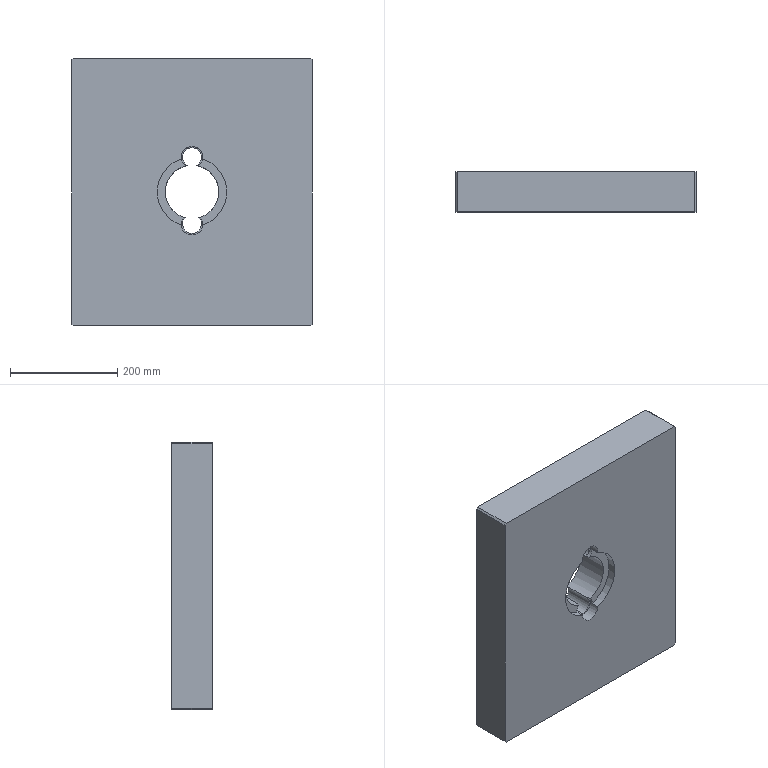Part | STEP file | 1 solid | 29 faces | box 450 x 75 x 500 mm | volume 16040639 mm3 | plane 19 | cylinder 10 | commonest cylinder face diameters 35 x3 40.5 x3 100 x2 130 x2